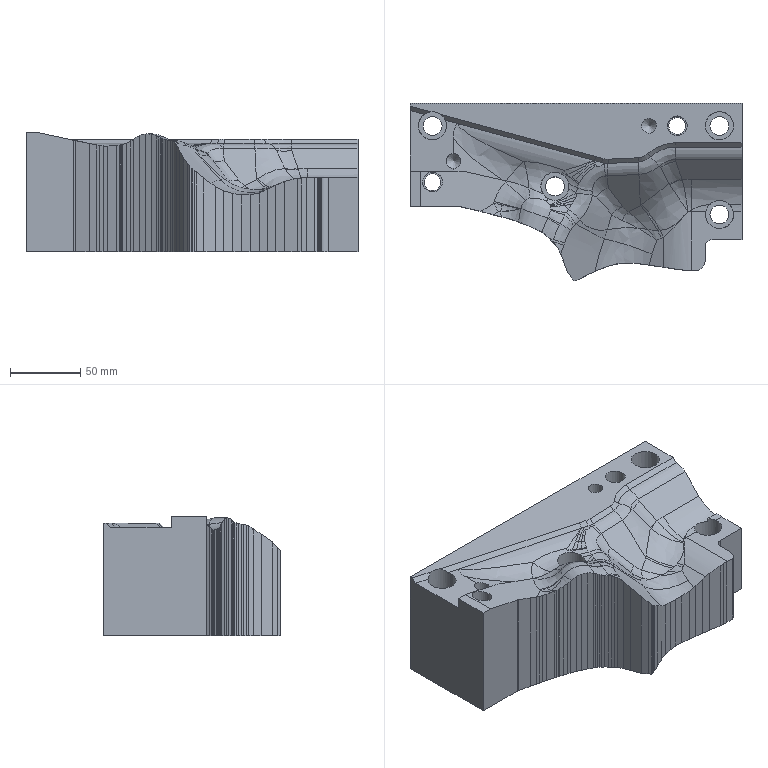Part | STEP file | lll_id5058_x_t | 1 solid | 223 faces | box 236 x 126.012 x 85 mm | volume 1511607 mm3 | spline 90 | plane 88 | cylinder 38 | torus 3 | cone 3 | sphere 1 | commonest cylinder face diameters 25 x5 65 x5 13.509 x4 20.008 x4 2 x2 10 x2